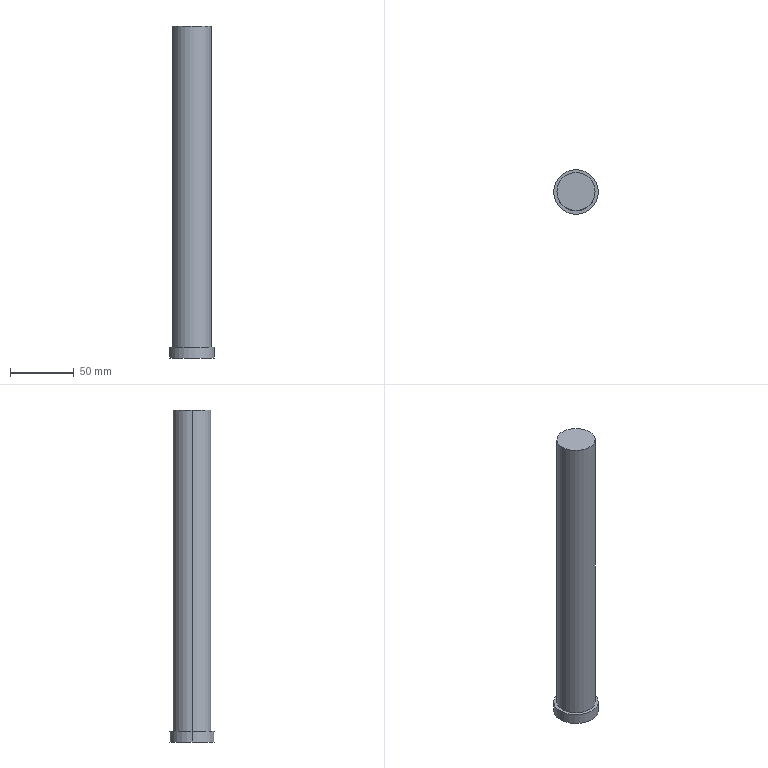Part | Creo | 1 solid | 7 faces | box 35 x 35 x 261 mm | volume 186660 mm3 | cylinder 4 | plane 3 | commonest cylinder face diameters 30 x2 35 x2
STEP:
#1=CARTESIAN_POINT('',(-175.,315.,0.5));
#2=VERTEX_POINT('',#1);
#3=CARTESIAN_POINT('',(-145.,315.,0.5));
#4=VERTEX_POINT('',#3);
#5=CARTESIAN_POINT('',(-160.,315.,0.5));
#6=DIRECTION('',(0.,0.,1.));
#7=DIRECTION('',(-1.,0.,0.));
#8=AXIS2_PLACEMENT_3D('',#5,#6,#7);
#9=CIRCLE('',#8,15.);
#10=EDGE_CURVE('',#2,#4,#9,.T.);
#11=ORIENTED_EDGE('',*,*,#10,.F.);
#12=CARTESIAN_POINT('',(-160.,315.,0.5));
#13=DIRECTION('',(0.,0.,1.));
#14=DIRECTION('',(1.,0.,0.));
#15=AXIS2_PLACEMENT_3D('',#12,#13,#14);
#16=CIRCLE('',#15,15.);
#17=EDGE_CURVE('',#4,#2,#16,.T.);
#18=ORIENTED_EDGE('',*,*,#17,.F.);
#19=EDGE_LOOP('',(#11,#18));
#20=FACE_OUTER_BOUND('',#19,.F.);
#21=CARTESIAN_POINT('',(-160.,315.,0.5));
#22=DIRECTION('',(0.,0.,1.));
#23=DIRECTION('',(1.,0.,0.));
#24=AXIS2_PLACEMENT_3D('',#21,#22,#23);
#25=PLANE('',#24);
#26=ADVANCED_FACE('',(#20),#25,.T.);
#27=CARTESIAN_POINT('',(-145.,315.,-252.));
#28=VERTEX_POINT('',#27);
#29=CARTESIAN_POINT('',(-175.,315.,-252.));
#30=VERTEX_POINT('',#29);
#31=CARTESIAN_POINT('',(-160.,315.,-252.));
#32=DIRECTION('',(0.,0.,-1.));
#33=DIRECTION('',(1.,0.,0.));
#34=AXIS2_PLACEMENT_3D('',#31,#32,#33);
#35=CIRCLE('',#34,15.);
#36=EDGE_CURVE('',#28,#30,#35,.T.);
#37=ORIENTED_EDGE('',*,*,#36,.T.);
#38=CARTESIAN_POINT('',(-175.,315.,-252.));
#39=DIRECTION('',(0.,0.,1.));
#40=VECTOR('',#39,252.5);
#41=LINE('',#38,#40);
#42=EDGE_CURVE('',#30,#2,#41,.T.);
#43=ORIENTED_EDGE('',*,*,#42,.T.);
#44=ORIENTED_EDGE('',*,*,#10,.T.);
#45=CARTESIAN_POINT('',(-145.,315.,-252.));
#46=DIRECTION('',(0.,0.,1.));
#47=VECTOR('',#46,252.5);
#48=LINE('',#45,#47);
#49=EDGE_CURVE('',#28,#4,#48,.T.);
#50=ORIENTED_EDGE('',*,*,#49,.F.);
#51=EDGE_LOOP('',(#37,#43,#44,#50));
#52=FACE_OUTER_BOUND('',#51,.F.);
#53=CARTESIAN_POINT('',(-160.,315.,-265.5));
#54=DIRECTION('',(0.,0.,1.));
#55=DIRECTION('',(1.,0.,0.));
#56=AXIS2_PLACEMENT_3D('',#53,#54,#55);
#57=CYLINDRICAL_SURFACE('',#56,15.);
#58=ADVANCED_FACE('',(#52),#57,.T.);
#59=CARTESIAN_POINT('',(-177.5,315.,-252.));
#60=VERTEX_POINT('',#59);
#61=CARTESIAN_POINT('',(-142.5,315.,-252.));
#62=VERTEX_POINT('',#61);
#63=CARTESIAN_POINT('',(-160.,315.,-252.));
#64=DIRECTION('',(0.,0.,1.));
#65=DIRECTION('',(-1.,0.,0.));
#66=AXIS2_PLACEMENT_3D('',#63,#64,#65);
#67=CIRCLE('',#66,17.5);
#68=EDGE_CURVE('',#60,#62,#67,.T.);
#69=ORIENTED_EDGE('',*,*,#68,.F.);
#70=CARTESIAN_POINT('',(-160.,315.,-252.));
#71=DIRECTION('',(0.,0.,1.));
#72=DIRECTION('',(1.,0.,0.));
#73=AXIS2_PLACEMENT_3D('',#70,#71,#72);
#74=CIRCLE('',#73,17.5);
#75=EDGE_CURVE('',#62,#60,#74,.T.);
#76=ORIENTED_EDGE('',*,*,#75,.F.);
#77=EDGE_LOOP('',(#69,#76));
#78=FACE_OUTER_BOUND('',#77,.F.);
#79=ORIENTED_EDGE('',*,*,#36,.F.);
#80=CARTESIAN_POINT('',(-160.,315.,-252.));
#81=DIRECTION('',(0.,0.,-1.));
#82=DIRECTION('',(-1.,0.,0.));
#83=AXIS2_PLACEMENT_3D('',#80,#81,#82);
#84=CIRCLE('',#83,15.);
#85=EDGE_CURVE('',#30,#28,#84,.T.);
#86=ORIENTED_EDGE('',*,*,#85,.F.);
#87=EDGE_LOOP('',(#79,#86));
#88=FACE_BOUND('',#87,.F.);
#89=CARTESIAN_POINT('',(-160.,315.,-252.));
#90=DIRECTION('',(0.,0.,1.));
#91=DIRECTION('',(1.,0.,0.));
#92=AXIS2_PLACEMENT_3D('',#89,#90,#91);
#93=PLANE('',#92);
#94=ADVANCED_FACE('',(#78,#88),#93,.T.);
#95=ORIENTED_EDGE('',*,*,#85,.T.);
#96=ORIENTED_EDGE('',*,*,#49,.T.);
#97=ORIENTED_EDGE('',*,*,#17,.T.);
#98=ORIENTED_EDGE('',*,*,#42,.F.);
#99=EDGE_LOOP('',(#95,#96,#97,#98));
#100=FACE_OUTER_BOUND('',#99,.F.);
#101=CARTESIAN_POINT('',(-160.,315.,-265.5));
#102=DIRECTION('',(0.,0.,1.));
#103=DIRECTION('',(1.,0.,0.));
#104=AXIS2_PLACEMENT_3D('',#101,#102,#103);
#105=CYLINDRICAL_SURFACE('',#104,15.);
#106=ADVANCED_FACE('',(#100),#105,.T.);
#107=ORIENTED_EDGE('',*,*,#68,.T.);
#108=CARTESIAN_POINT('',(-142.5,315.,-260.5));
#109=VERTEX_POINT('',#108);
#110=CARTESIAN_POINT('',(-142.5,315.,-260.5));
#111=DIRECTION('',(0.,0.,1.));
#112=VECTOR('',#111,8.5);
#113=LINE('',#110,#112);
#114=EDGE_CURVE('',#109,#62,#113,.T.);
#115=ORIENTED_EDGE('',*,*,#114,.F.);
#116=CARTESIAN_POINT('',(-177.5,315.,-260.5));
#117=VERTEX_POINT('',#116);
#118=CARTESIAN_POINT('',(-160.,315.,-260.5));
#119=DIRECTION('',(0.,0.,-1.));
#120=DIRECTION('',(1.,0.,0.));
#121=AXIS2_PLACEMENT_3D('',#118,#119,#120);
#122=CIRCLE('',#121,17.5);
#123=EDGE_CURVE('',#109,#117,#122,.T.);
#124=ORIENTED_EDGE('',*,*,#123,.T.);
#125=CARTESIAN_POINT('',(-177.5,315.,-260.5));
#126=DIRECTION('',(0.,0.,1.));
#127=VECTOR('',#126,8.5);
#128=LINE('',#125,#127);
#129=EDGE_CURVE('',#117,#60,#128,.T.);
#130=ORIENTED_EDGE('',*,*,#129,.T.);
#131=EDGE_LOOP('',(#107,#115,#124,#130));
#132=FACE_OUTER_BOUND('',#131,.F.);
#133=CARTESIAN_POINT('',(-160.,315.,-260.5));
#134=DIRECTION('',(0.,0.,1.));
#135=DIRECTION('',(1.,0.,0.));
#136=AXIS2_PLACEMENT_3D('',#133,#134,#135);
#137=CYLINDRICAL_SURFACE('',#136,17.5);
#138=ADVANCED_FACE('',(#132),#137,.T.);
#139=ORIENTED_EDGE('',*,*,#75,.T.);
#140=ORIENTED_EDGE('',*,*,#129,.F.);
#141=CARTESIAN_POINT('',(-160.,315.,-260.5));
#142=DIRECTION('',(0.,0.,-1.));
#143=DIRECTION('',(-1.,0.,0.));
#144=AXIS2_PLACEMENT_3D('',#141,#142,#143);
#145=CIRCLE('',#144,17.5);
#146=EDGE_CURVE('',#117,#109,#145,.T.);
#147=ORIENTED_EDGE('',*,*,#146,.T.);
#148=ORIENTED_EDGE('',*,*,#114,.T.);
#149=EDGE_LOOP('',(#139,#140,#147,#148));
#150=FACE_OUTER_BOUND('',#149,.F.);
#151=CARTESIAN_POINT('',(-160.,315.,-260.5));
#152=DIRECTION('',(0.,0.,1.));
#153=DIRECTION('',(1.,0.,0.));
#154=AXIS2_PLACEMENT_3D('',#151,#152,#153);
#155=CYLINDRICAL_SURFACE('',#154,17.5);
#156=ADVANCED_FACE('',(#150),#155,.T.);
#157=ORIENTED_EDGE('',*,*,#123,.F.);
#158=ORIENTED_EDGE('',*,*,#146,.F.);
#159=EDGE_LOOP('',(#157,#158));
#160=FACE_OUTER_BOUND('',#159,.F.);
#161=CARTESIAN_POINT('',(-160.,315.,-260.5));
#162=DIRECTION('',(0.,0.,-1.));
#163=DIRECTION('',(-1.,0.,0.));
#164=AXIS2_PLACEMENT_3D('',#161,#162,#163);
#165=PLANE('',#164);
#166=ADVANCED_FACE('',(#160),#165,.T.);
#167=CLOSED_SHELL('',(#26,#58,#94,#106,#138,#156,#166));
#168=MANIFOLD_SOLID_BREP('',#167);
#169=(LENGTH_UNIT()NAMED_UNIT(*)SI_UNIT(.MILLI.,.METRE.));
#170=UNCERTAINTY_MEASURE_WITH_UNIT(LENGTH_MEASURE(0.02656),#169,'','');
#171=(NAMED_UNIT(*)PLANE_ANGLE_UNIT()SI_UNIT($,.RADIAN.));
#172=PLANE_ANGLE_MEASURE_WITH_UNIT(PLANE_ANGLE_MEASURE(0.01745),#171);
#173=(CONVERSION_BASED_UNIT('DEGREE',#172)NAMED_UNIT(*)PLANE_ANGLE_UNIT());
#174=(NAMED_UNIT(*)SI_UNIT($,.STERADIAN.)SOLID_ANGLE_UNIT());
#175=(GEOMETRIC_REPRESENTATION_CONTEXT(3)GLOBAL_UNCERTAINTY_ASSIGNED_CONTEXT((#170))GLOBAL_UNIT_ASSIGNED_CONTEXT((#169,#173,#174))REPRESENTATION_CONTEXT('',''));
#176=ADVANCED_BREP_SHAPE_REPRESENTATION('',(#168),#175);